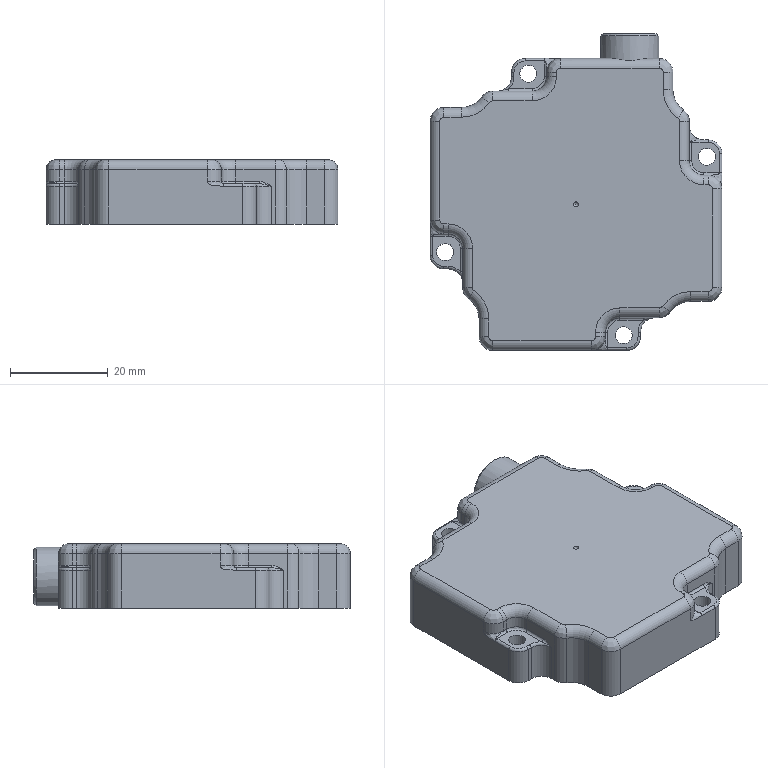Part | STEP file | 1 solid | 138 faces | box 59.8 x 64.9 x 13.2 mm | volume 38412 mm3 | cylinder 66 | plane 28 | spline 23 | torus 19 | cone 1 | sphere 1 | commonest cylinder face diameters 1 x16 4 x16 5.6 x16 6 x8 3.5 x4 10 x4